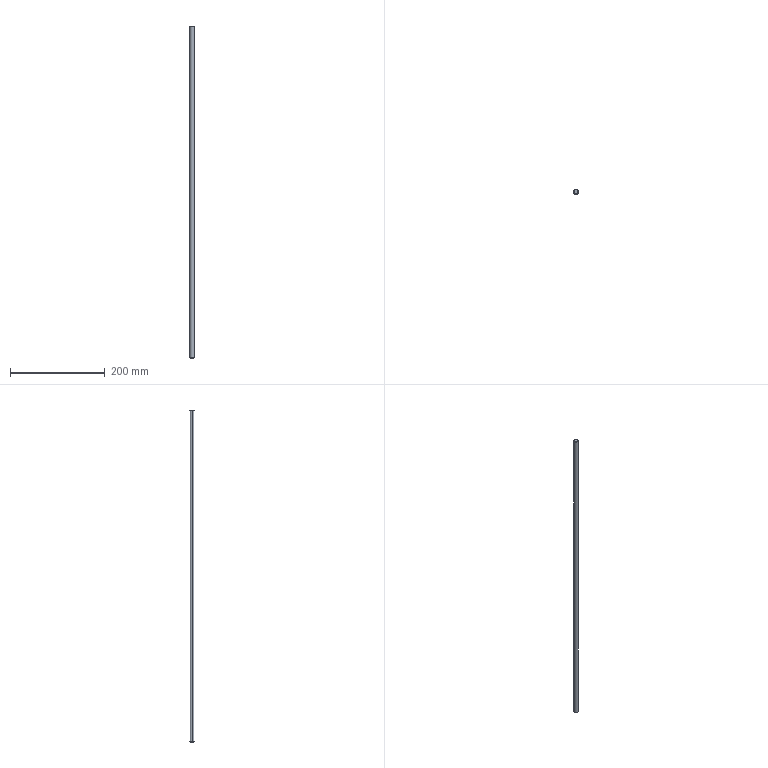Part | SolidWorks | features Chamfer 1, Extrusion 1 | 1 solid | 8 faces | box 10 x 10 x 700 mm | volume 54949 mm3 | cone 4 | cylinder 2 | plane 2 | commonest cylinder face diameters 10 x2
STEP:
#1=CARTESIAN_POINT('',(-4.,0.,-350.));
#2=VERTEX_POINT('',#1);
#3=CARTESIAN_POINT('',(4.,0.,-350.));
#4=VERTEX_POINT('',#3);
#5=CARTESIAN_POINT('',(0.,0.,-350.));
#6=DIRECTION('',(0.,0.,-1.));
#7=DIRECTION('',(1.,0.,0.));
#8=AXIS2_PLACEMENT_3D('',#5,#6,#7);
#9=CIRCLE('',#8,4.);
#10=EDGE_CURVE('',#2,#4,#9,.T.);
#11=ORIENTED_EDGE('',*,*,#10,.F.);
#12=CARTESIAN_POINT('',(-5.,0.,-349.));
#13=VERTEX_POINT('',#12);
#14=CARTESIAN_POINT('',(-5.,0.,-349.));
#15=DIRECTION('',(-0.7071,0.,0.7071));
#16=VECTOR('',#15,1000.);
#17=LINE('',#14,#16);
#18=EDGE_CURVE('',#2,#13,#17,.T.);
#19=ORIENTED_EDGE('',*,*,#18,.T.);
#20=CARTESIAN_POINT('',(5.,0.,-349.));
#21=VERTEX_POINT('',#20);
#22=CARTESIAN_POINT('',(0.,0.,-349.));
#23=DIRECTION('',(0.,0.,1.));
#24=DIRECTION('',(1.,0.,0.));
#25=AXIS2_PLACEMENT_3D('',#22,#23,#24);
#26=CIRCLE('',#25,5.);
#27=EDGE_CURVE('',#21,#13,#26,.T.);
#28=ORIENTED_EDGE('',*,*,#27,.F.);
#29=CARTESIAN_POINT('',(5.,0.,-349.));
#30=DIRECTION('',(0.7071,0.,0.7071));
#31=VECTOR('',#30,1000.);
#32=LINE('',#29,#31);
#33=EDGE_CURVE('',#4,#21,#32,.T.);
#34=ORIENTED_EDGE('',*,*,#33,.F.);
#35=EDGE_LOOP('',(#11,#19,#28,#34));
#36=FACE_OUTER_BOUND('',#35,.T.);
#37=CARTESIAN_POINT('',(0.,0.,-349.));
#38=DIRECTION('',(0.,0.,1.));
#39=DIRECTION('',(1.,0.,0.));
#40=AXIS2_PLACEMENT_3D('',#37,#38,#39);
#41=CONICAL_SURFACE('',#40,5.,0.7854);
#42=ADVANCED_FACE('',(#36),#41,.T.);
#43=CARTESIAN_POINT('',(4.,0.,350.));
#44=VERTEX_POINT('',#43);
#45=CARTESIAN_POINT('',(-4.,0.,350.));
#46=VERTEX_POINT('',#45);
#47=CARTESIAN_POINT('',(0.,0.,350.));
#48=DIRECTION('',(0.,0.,1.));
#49=DIRECTION('',(1.,0.,0.));
#50=AXIS2_PLACEMENT_3D('',#47,#48,#49);
#51=CIRCLE('',#50,4.);
#52=EDGE_CURVE('',#44,#46,#51,.T.);
#53=ORIENTED_EDGE('',*,*,#52,.F.);
#54=CARTESIAN_POINT('',(5.,0.,349.));
#55=VERTEX_POINT('',#54);
#56=CARTESIAN_POINT('',(4.,0.,350.));
#57=DIRECTION('',(0.7071,0.,-0.7071));
#58=VECTOR('',#57,1000.);
#59=LINE('',#56,#58);
#60=EDGE_CURVE('',#44,#55,#59,.T.);
#61=ORIENTED_EDGE('',*,*,#60,.T.);
#62=CARTESIAN_POINT('',(-5.,0.,349.));
#63=VERTEX_POINT('',#62);
#64=CARTESIAN_POINT('',(0.,0.,349.));
#65=DIRECTION('',(0.,0.,-1.));
#66=DIRECTION('',(1.,0.,0.));
#67=AXIS2_PLACEMENT_3D('',#64,#65,#66);
#68=CIRCLE('',#67,5.);
#69=EDGE_CURVE('',#63,#55,#68,.T.);
#70=ORIENTED_EDGE('',*,*,#69,.F.);
#71=CARTESIAN_POINT('',(-4.,0.,350.));
#72=DIRECTION('',(-0.7071,0.,-0.7071));
#73=VECTOR('',#72,1000.);
#74=LINE('',#71,#73);
#75=EDGE_CURVE('',#46,#63,#74,.T.);
#76=ORIENTED_EDGE('',*,*,#75,.F.);
#77=EDGE_LOOP('',(#53,#61,#70,#76));
#78=FACE_OUTER_BOUND('',#77,.T.);
#79=CARTESIAN_POINT('',(0.,0.,350.));
#80=DIRECTION('',(0.,0.,-1.));
#81=DIRECTION('',(-1.,0.,0.));
#82=AXIS2_PLACEMENT_3D('',#79,#80,#81);
#83=CONICAL_SURFACE('',#82,4.,0.7854);
#84=ADVANCED_FACE('',(#78),#83,.T.);
#85=ORIENTED_EDGE('',*,*,#69,.T.);
#86=CARTESIAN_POINT('',(5.,0.,350.));
#87=DIRECTION('',(0.,0.,-1.));
#88=VECTOR('',#87,1000.);
#89=LINE('',#86,#88);
#90=EDGE_CURVE('',#55,#21,#89,.T.);
#91=ORIENTED_EDGE('',*,*,#90,.T.);
#92=ORIENTED_EDGE('',*,*,#27,.T.);
#93=CARTESIAN_POINT('',(-5.,0.,350.));
#94=DIRECTION('',(0.,0.,-1.));
#95=VECTOR('',#94,1000.);
#96=LINE('',#93,#95);
#97=EDGE_CURVE('',#63,#13,#96,.T.);
#98=ORIENTED_EDGE('',*,*,#97,.F.);
#99=EDGE_LOOP('',(#85,#91,#92,#98));
#100=FACE_OUTER_BOUND('',#99,.T.);
#101=CARTESIAN_POINT('',(0.,0.,350.));
#102=DIRECTION('',(0.,0.,-1.));
#103=DIRECTION('',(-1.,0.,0.));
#104=AXIS2_PLACEMENT_3D('',#101,#102,#103);
#105=CYLINDRICAL_SURFACE('',#104,5.);
#106=ADVANCED_FACE('',(#100),#105,.T.);
#107=ORIENTED_EDGE('',*,*,#90,.F.);
#108=CARTESIAN_POINT('',(0.,0.,349.));
#109=DIRECTION('',(0.,0.,-1.));
#110=DIRECTION('',(1.,0.,0.));
#111=AXIS2_PLACEMENT_3D('',#108,#109,#110);
#112=CIRCLE('',#111,5.);
#113=EDGE_CURVE('',#55,#63,#112,.T.);
#114=ORIENTED_EDGE('',*,*,#113,.T.);
#115=ORIENTED_EDGE('',*,*,#97,.T.);
#116=CARTESIAN_POINT('',(0.,0.,-349.));
#117=DIRECTION('',(0.,0.,1.));
#118=DIRECTION('',(1.,0.,0.));
#119=AXIS2_PLACEMENT_3D('',#116,#117,#118);
#120=CIRCLE('',#119,5.);
#121=EDGE_CURVE('',#13,#21,#120,.T.);
#122=ORIENTED_EDGE('',*,*,#121,.T.);
#123=EDGE_LOOP('',(#107,#114,#115,#122));
#124=FACE_OUTER_BOUND('',#123,.T.);
#125=CARTESIAN_POINT('',(0.,0.,350.));
#126=DIRECTION('',(0.,0.,-1.));
#127=DIRECTION('',(-1.,0.,0.));
#128=AXIS2_PLACEMENT_3D('',#125,#126,#127);
#129=CYLINDRICAL_SURFACE('',#128,5.);
#130=ADVANCED_FACE('',(#124),#129,.T.);
#131=CARTESIAN_POINT('',(0.,0.,350.));
#132=DIRECTION('',(0.,0.,1.));
#133=DIRECTION('',(1.,0.,0.));
#134=AXIS2_PLACEMENT_3D('',#131,#132,#133);
#135=CIRCLE('',#134,4.);
#136=EDGE_CURVE('',#46,#44,#135,.T.);
#137=ORIENTED_EDGE('',*,*,#136,.T.);
#138=ORIENTED_EDGE('',*,*,#52,.T.);
#139=EDGE_LOOP('',(#137,#138));
#140=FACE_OUTER_BOUND('',#139,.T.);
#141=CARTESIAN_POINT('',(0.,0.,350.));
#142=DIRECTION('',(0.,0.,1.));
#143=DIRECTION('',(1.,0.,0.));
#144=AXIS2_PLACEMENT_3D('',#141,#142,#143);
#145=PLANE('',#144);
#146=ADVANCED_FACE('',(#140),#145,.T.);
#147=CARTESIAN_POINT('',(0.,0.,-350.));
#148=DIRECTION('',(0.,0.,-1.));
#149=DIRECTION('',(1.,0.,0.));
#150=AXIS2_PLACEMENT_3D('',#147,#148,#149);
#151=CIRCLE('',#150,4.);
#152=EDGE_CURVE('',#4,#2,#151,.T.);
#153=ORIENTED_EDGE('',*,*,#152,.T.);
#154=ORIENTED_EDGE('',*,*,#10,.T.);
#155=EDGE_LOOP('',(#153,#154));
#156=FACE_OUTER_BOUND('',#155,.T.);
#157=CARTESIAN_POINT('',(0.,0.,-350.));
#158=DIRECTION('',(0.,0.,1.));
#159=DIRECTION('',(1.,0.,0.));
#160=AXIS2_PLACEMENT_3D('',#157,#158,#159);
#161=PLANE('',#160);
#162=ADVANCED_FACE('',(#156),#161,.F.);
#163=ORIENTED_EDGE('',*,*,#60,.F.);
#164=ORIENTED_EDGE('',*,*,#136,.F.);
#165=ORIENTED_EDGE('',*,*,#75,.T.);
#166=ORIENTED_EDGE('',*,*,#113,.F.);
#167=EDGE_LOOP('',(#163,#164,#165,#166));
#168=FACE_OUTER_BOUND('',#167,.T.);
#169=CARTESIAN_POINT('',(0.,0.,350.));
#170=DIRECTION('',(0.,0.,-1.));
#171=DIRECTION('',(-1.,0.,0.));
#172=AXIS2_PLACEMENT_3D('',#169,#170,#171);
#173=CONICAL_SURFACE('',#172,4.,0.7854);
#174=ADVANCED_FACE('',(#168),#173,.T.);
#175=ORIENTED_EDGE('',*,*,#18,.F.);
#176=ORIENTED_EDGE('',*,*,#152,.F.);
#177=ORIENTED_EDGE('',*,*,#33,.T.);
#178=ORIENTED_EDGE('',*,*,#121,.F.);
#179=EDGE_LOOP('',(#175,#176,#177,#178));
#180=FACE_OUTER_BOUND('',#179,.T.);
#181=CARTESIAN_POINT('',(0.,0.,-349.));
#182=DIRECTION('',(0.,0.,1.));
#183=DIRECTION('',(1.,0.,0.));
#184=AXIS2_PLACEMENT_3D('',#181,#182,#183);
#185=CONICAL_SURFACE('',#184,5.,0.7854);
#186=ADVANCED_FACE('',(#180),#185,.T.);
#187=CLOSED_SHELL('',(#42,#84,#106,#130,#146,#162,#174,#186));
#188=MANIFOLD_SOLID_BREP('',#187);
#189=CARTESIAN_POINT('',(0.,0.,0.));
#190=DIRECTION('',(0.,0.,1.));
#191=DIRECTION('',(1.,0.,0.));
#192=AXIS2_PLACEMENT_3D('',#189,#190,#191);
#193=(LENGTH_UNIT()NAMED_UNIT(*)SI_UNIT(.MILLI.,.METRE.));
#194=UNCERTAINTY_MEASURE_WITH_UNIT(LENGTH_MEASURE(0.00001),#193,'','');
#195=(NAMED_UNIT(*)PLANE_ANGLE_UNIT()SI_UNIT($,.RADIAN.));
#196=(NAMED_UNIT(*)SI_UNIT($,.STERADIAN.)SOLID_ANGLE_UNIT());
#197=(GEOMETRIC_REPRESENTATION_CONTEXT(3)GLOBAL_UNCERTAINTY_ASSIGNED_CONTEXT((#194))GLOBAL_UNIT_ASSIGNED_CONTEXT((#193,#195,#196))REPRESENTATION_CONTEXT('',''));
#198=ADVANCED_BREP_SHAPE_REPRESENTATION('',(#188,#192),#197);